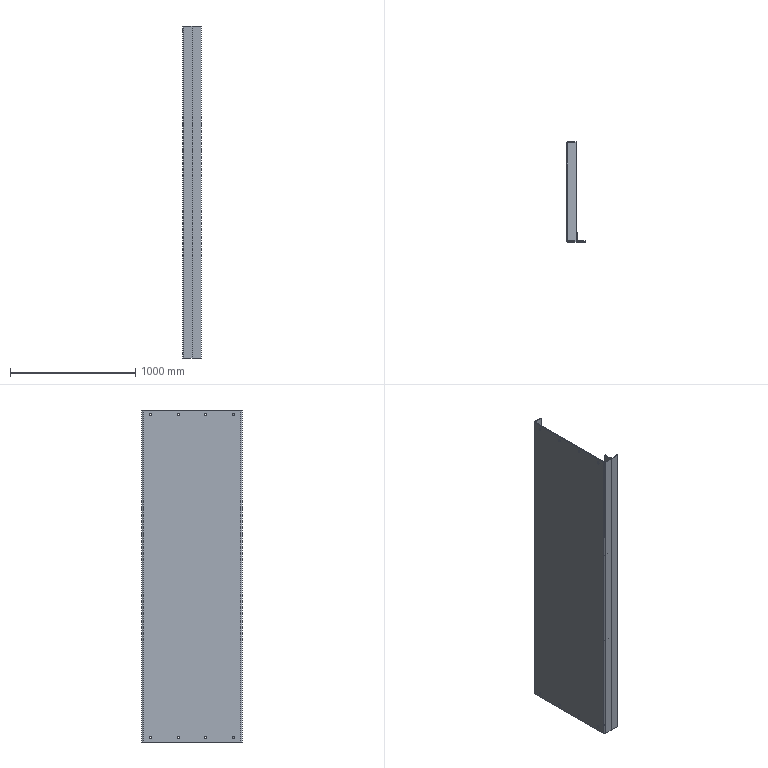Part | STEP file | Rear baffle_Default<As machined> | 6 solids | 81 faces | box 150 x 800 x 2650 mm | volume 24404542 mm3 | plane 50 | cylinder 31 | commonest cylinder face diameters 18 x17 4 x10 5.333 x2 20 x2